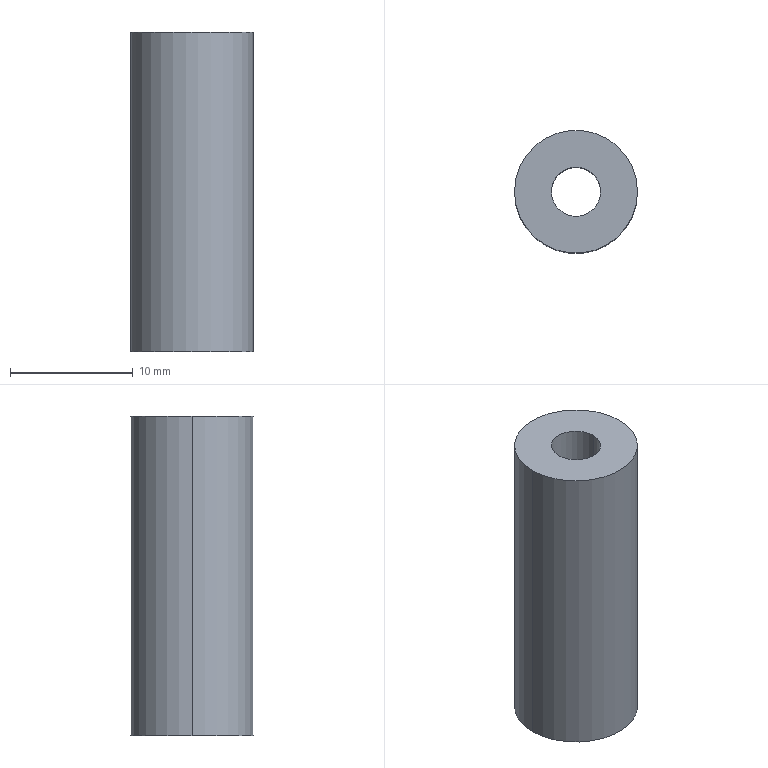Part | SolidWorks | features Extrusion 1 | 1 solid | 6 faces | box 10 x 10 x 26 mm | volume 1715 mm3 | cylinder 4 | plane 2 | commonest cylinder face diameters 4 x2 10 x2
STEP:
#1=CARTESIAN_POINT('',(-2.,0.,-13.));
#2=VERTEX_POINT('',#1);
#3=CARTESIAN_POINT('',(2.,0.,-13.));
#4=VERTEX_POINT('',#3);
#5=CARTESIAN_POINT('',(0.,0.,-13.));
#6=DIRECTION('',(0.,0.,1.));
#7=DIRECTION('',(1.,0.,0.));
#8=AXIS2_PLACEMENT_3D('',#5,#6,#7);
#9=CIRCLE('',#8,2.);
#10=EDGE_CURVE('',#2,#4,#9,.T.);
#11=ORIENTED_EDGE('',*,*,#10,.F.);
#12=CARTESIAN_POINT('',(-2.,0.,13.));
#13=VERTEX_POINT('',#12);
#14=CARTESIAN_POINT('',(-2.,0.,-13.));
#15=DIRECTION('',(0.,0.,1.));
#16=VECTOR('',#15,1000.);
#17=LINE('',#14,#16);
#18=EDGE_CURVE('',#2,#13,#17,.T.);
#19=ORIENTED_EDGE('',*,*,#18,.T.);
#20=CARTESIAN_POINT('',(2.,0.,13.));
#21=VERTEX_POINT('',#20);
#22=CARTESIAN_POINT('',(0.,0.,13.));
#23=DIRECTION('',(0.,0.,1.));
#24=DIRECTION('',(1.,0.,0.));
#25=AXIS2_PLACEMENT_3D('',#22,#23,#24);
#26=CIRCLE('',#25,2.);
#27=EDGE_CURVE('',#13,#21,#26,.T.);
#28=ORIENTED_EDGE('',*,*,#27,.T.);
#29=CARTESIAN_POINT('',(2.,0.,-13.));
#30=DIRECTION('',(0.,0.,1.));
#31=VECTOR('',#30,1000.);
#32=LINE('',#29,#31);
#33=EDGE_CURVE('',#4,#21,#32,.T.);
#34=ORIENTED_EDGE('',*,*,#33,.F.);
#35=EDGE_LOOP('',(#11,#19,#28,#34));
#36=FACE_OUTER_BOUND('',#35,.T.);
#37=CARTESIAN_POINT('',(0.,0.,-13.));
#38=DIRECTION('',(0.,0.,1.));
#39=DIRECTION('',(1.,0.,0.));
#40=AXIS2_PLACEMENT_3D('',#37,#38,#39);
#41=CYLINDRICAL_SURFACE('',#40,2.);
#42=ADVANCED_FACE('',(#36),#41,.F.);
#43=CARTESIAN_POINT('',(5.,0.,-13.));
#44=VERTEX_POINT('',#43);
#45=CARTESIAN_POINT('',(-5.,0.,-13.));
#46=VERTEX_POINT('',#45);
#47=CARTESIAN_POINT('',(0.,0.,-13.));
#48=DIRECTION('',(0.,0.,1.));
#49=DIRECTION('',(1.,0.,0.));
#50=AXIS2_PLACEMENT_3D('',#47,#48,#49);
#51=CIRCLE('',#50,5.);
#52=EDGE_CURVE('',#44,#46,#51,.T.);
#53=ORIENTED_EDGE('',*,*,#52,.T.);
#54=CARTESIAN_POINT('',(-5.,0.,13.));
#55=VERTEX_POINT('',#54);
#56=CARTESIAN_POINT('',(-5.,0.,-13.));
#57=DIRECTION('',(0.,0.,1.));
#58=VECTOR('',#57,1000.);
#59=LINE('',#56,#58);
#60=EDGE_CURVE('',#46,#55,#59,.T.);
#61=ORIENTED_EDGE('',*,*,#60,.T.);
#62=CARTESIAN_POINT('',(5.,0.,13.));
#63=VERTEX_POINT('',#62);
#64=CARTESIAN_POINT('',(0.,0.,13.));
#65=DIRECTION('',(0.,0.,1.));
#66=DIRECTION('',(1.,0.,0.));
#67=AXIS2_PLACEMENT_3D('',#64,#65,#66);
#68=CIRCLE('',#67,5.);
#69=EDGE_CURVE('',#63,#55,#68,.T.);
#70=ORIENTED_EDGE('',*,*,#69,.F.);
#71=CARTESIAN_POINT('',(5.,0.,-13.));
#72=DIRECTION('',(0.,0.,1.));
#73=VECTOR('',#72,1000.);
#74=LINE('',#71,#73);
#75=EDGE_CURVE('',#44,#63,#74,.T.);
#76=ORIENTED_EDGE('',*,*,#75,.F.);
#77=EDGE_LOOP('',(#53,#61,#70,#76));
#78=FACE_OUTER_BOUND('',#77,.T.);
#79=CARTESIAN_POINT('',(0.,0.,-13.));
#80=DIRECTION('',(0.,0.,1.));
#81=DIRECTION('',(1.,0.,0.));
#82=AXIS2_PLACEMENT_3D('',#79,#80,#81);
#83=CYLINDRICAL_SURFACE('',#82,5.);
#84=ADVANCED_FACE('',(#78),#83,.T.);
#85=ORIENTED_EDGE('',*,*,#60,.F.);
#86=CARTESIAN_POINT('',(0.,0.,-13.));
#87=DIRECTION('',(0.,0.,1.));
#88=DIRECTION('',(1.,0.,0.));
#89=AXIS2_PLACEMENT_3D('',#86,#87,#88);
#90=CIRCLE('',#89,5.);
#91=EDGE_CURVE('',#46,#44,#90,.T.);
#92=ORIENTED_EDGE('',*,*,#91,.T.);
#93=ORIENTED_EDGE('',*,*,#75,.T.);
#94=CARTESIAN_POINT('',(0.,0.,13.));
#95=DIRECTION('',(0.,0.,1.));
#96=DIRECTION('',(1.,0.,0.));
#97=AXIS2_PLACEMENT_3D('',#94,#95,#96);
#98=CIRCLE('',#97,5.);
#99=EDGE_CURVE('',#55,#63,#98,.T.);
#100=ORIENTED_EDGE('',*,*,#99,.F.);
#101=EDGE_LOOP('',(#85,#92,#93,#100));
#102=FACE_OUTER_BOUND('',#101,.T.);
#103=CARTESIAN_POINT('',(0.,0.,-13.));
#104=DIRECTION('',(0.,0.,1.));
#105=DIRECTION('',(1.,0.,0.));
#106=AXIS2_PLACEMENT_3D('',#103,#104,#105);
#107=CYLINDRICAL_SURFACE('',#106,5.);
#108=ADVANCED_FACE('',(#102),#107,.T.);
#109=CARTESIAN_POINT('',(0.,0.,-13.));
#110=DIRECTION('',(0.,0.,1.));
#111=DIRECTION('',(1.,0.,0.));
#112=AXIS2_PLACEMENT_3D('',#109,#110,#111);
#113=CIRCLE('',#112,2.);
#114=EDGE_CURVE('',#4,#2,#113,.T.);
#115=ORIENTED_EDGE('',*,*,#114,.T.);
#116=ORIENTED_EDGE('',*,*,#10,.T.);
#117=EDGE_LOOP('',(#115,#116));
#118=FACE_BOUND('',#117,.T.);
#119=ORIENTED_EDGE('',*,*,#52,.F.);
#120=ORIENTED_EDGE('',*,*,#91,.F.);
#121=EDGE_LOOP('',(#119,#120));
#122=FACE_OUTER_BOUND('',#121,.T.);
#123=CARTESIAN_POINT('',(0.,0.,-13.));
#124=DIRECTION('',(0.,0.,1.));
#125=DIRECTION('',(1.,0.,0.));
#126=AXIS2_PLACEMENT_3D('',#123,#124,#125);
#127=PLANE('',#126);
#128=ADVANCED_FACE('',(#118,#122),#127,.F.);
#129=CARTESIAN_POINT('',(0.,0.,13.));
#130=DIRECTION('',(0.,0.,1.));
#131=DIRECTION('',(1.,0.,0.));
#132=AXIS2_PLACEMENT_3D('',#129,#130,#131);
#133=CIRCLE('',#132,2.);
#134=EDGE_CURVE('',#21,#13,#133,.T.);
#135=ORIENTED_EDGE('',*,*,#134,.F.);
#136=ORIENTED_EDGE('',*,*,#27,.F.);
#137=EDGE_LOOP('',(#135,#136));
#138=FACE_BOUND('',#137,.T.);
#139=ORIENTED_EDGE('',*,*,#69,.T.);
#140=ORIENTED_EDGE('',*,*,#99,.T.);
#141=EDGE_LOOP('',(#139,#140));
#142=FACE_OUTER_BOUND('',#141,.T.);
#143=CARTESIAN_POINT('',(0.,0.,13.));
#144=DIRECTION('',(0.,0.,1.));
#145=DIRECTION('',(1.,0.,0.));
#146=AXIS2_PLACEMENT_3D('',#143,#144,#145);
#147=PLANE('',#146);
#148=ADVANCED_FACE('',(#138,#142),#147,.T.);
#149=ORIENTED_EDGE('',*,*,#18,.F.);
#150=ORIENTED_EDGE('',*,*,#114,.F.);
#151=ORIENTED_EDGE('',*,*,#33,.T.);
#152=ORIENTED_EDGE('',*,*,#134,.T.);
#153=EDGE_LOOP('',(#149,#150,#151,#152));
#154=FACE_OUTER_BOUND('',#153,.T.);
#155=CARTESIAN_POINT('',(0.,0.,-13.));
#156=DIRECTION('',(0.,0.,1.));
#157=DIRECTION('',(1.,0.,0.));
#158=AXIS2_PLACEMENT_3D('',#155,#156,#157);
#159=CYLINDRICAL_SURFACE('',#158,2.);
#160=ADVANCED_FACE('',(#154),#159,.F.);
#161=CLOSED_SHELL('',(#42,#84,#108,#128,#148,#160));
#162=MANIFOLD_SOLID_BREP('',#161);
#163=CARTESIAN_POINT('',(0.,0.,0.));
#164=DIRECTION('',(0.,0.,1.));
#165=DIRECTION('',(1.,0.,0.));
#166=AXIS2_PLACEMENT_3D('',#163,#164,#165);
#167=(LENGTH_UNIT()NAMED_UNIT(*)SI_UNIT(.MILLI.,.METRE.));
#168=UNCERTAINTY_MEASURE_WITH_UNIT(LENGTH_MEASURE(0.00001),#167,'','');
#169=(NAMED_UNIT(*)PLANE_ANGLE_UNIT()SI_UNIT($,.RADIAN.));
#170=(NAMED_UNIT(*)SI_UNIT($,.STERADIAN.)SOLID_ANGLE_UNIT());
#171=(GEOMETRIC_REPRESENTATION_CONTEXT(3)GLOBAL_UNCERTAINTY_ASSIGNED_CONTEXT((#168))GLOBAL_UNIT_ASSIGNED_CONTEXT((#167,#169,#170))REPRESENTATION_CONTEXT('',''));
#172=ADVANCED_BREP_SHAPE_REPRESENTATION('',(#162,#166),#171);